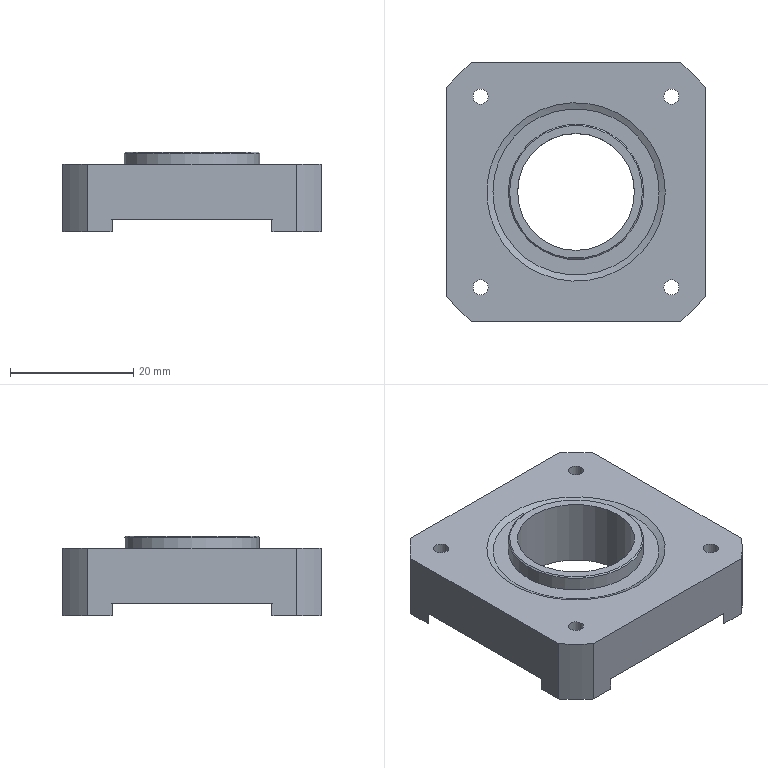Part | NX | 1 solid | 28 faces | box 42 x 42 x 13 mm | volume 13151 mm3 | plane 16 | cylinder 10 | cone 2 | commonest cylinder face diameters 2.459 x4 54 x4 19 x1 22 x1
STEP:
#1=CARTESIAN_POINT('',(-9.5,0.,2.));
#2=VERTEX_POINT('',#1);
#3=CARTESIAN_POINT('',(0.,0.,2.));
#4=DIRECTION('',(0.,0.,-1.));
#5=DIRECTION('',(-1.,0.,0.));
#6=AXIS2_PLACEMENT_3D('',#3,#4,#5);
#7=CIRCLE('',#6,9.5);
#8=EDGE_CURVE('',#2,#2,#7,.T.);
#9=ORIENTED_EDGE('',*,*,#8,.F.);
#10=EDGE_LOOP('',(#9));
#11=FACE_BOUND('',#10,.T.);
#12=CARTESIAN_POINT('',(16.73,-15.5,2.));
#13=VERTEX_POINT('',#12);
#14=CARTESIAN_POINT('',(15.5,-15.5,2.));
#15=DIRECTION('',(0.,0.,1.));
#16=DIRECTION('',(1.,0.,0.));
#17=AXIS2_PLACEMENT_3D('',#14,#15,#16);
#18=CIRCLE('',#17,1.23);
#19=EDGE_CURVE('',#13,#13,#18,.F.);
#20=ORIENTED_EDGE('',*,*,#19,.F.);
#21=EDGE_LOOP('',(#20));
#22=FACE_BOUND('',#21,.T.);
#23=CARTESIAN_POINT('',(-14.271,-15.5,2.));
#24=VERTEX_POINT('',#23);
#25=CARTESIAN_POINT('',(-15.5,-15.5,2.));
#26=DIRECTION('',(0.,0.,1.));
#27=DIRECTION('',(1.,0.,0.));
#28=AXIS2_PLACEMENT_3D('',#25,#26,#27);
#29=CIRCLE('',#28,1.23);
#30=EDGE_CURVE('',#24,#24,#29,.F.);
#31=ORIENTED_EDGE('',*,*,#30,.F.);
#32=EDGE_LOOP('',(#31));
#33=FACE_BOUND('',#32,.T.);
#34=CARTESIAN_POINT('',(16.73,15.5,2.));
#35=VERTEX_POINT('',#34);
#36=CARTESIAN_POINT('',(15.5,15.5,2.));
#37=DIRECTION('',(0.,0.,1.));
#38=DIRECTION('',(1.,0.,0.));
#39=AXIS2_PLACEMENT_3D('',#36,#37,#38);
#40=CIRCLE('',#39,1.23);
#41=EDGE_CURVE('',#35,#35,#40,.F.);
#42=ORIENTED_EDGE('',*,*,#41,.F.);
#43=EDGE_LOOP('',(#42));
#44=FACE_BOUND('',#43,.T.);
#45=CARTESIAN_POINT('',(-14.271,15.5,2.));
#46=VERTEX_POINT('',#45);
#47=CARTESIAN_POINT('',(-15.5,15.5,2.));
#48=DIRECTION('',(0.,0.,1.));
#49=DIRECTION('',(1.,0.,0.));
#50=AXIS2_PLACEMENT_3D('',#47,#48,#49);
#51=CIRCLE('',#50,1.23);
#52=EDGE_CURVE('',#46,#46,#51,.F.);
#53=ORIENTED_EDGE('',*,*,#52,.F.);
#54=EDGE_LOOP('',(#53));
#55=FACE_BOUND('',#54,.T.);
#56=CARTESIAN_POINT('',(13.,-21.,2.));
#57=VERTEX_POINT('',#56);
#58=CARTESIAN_POINT('',(21.,-13.,2.));
#59=VERTEX_POINT('',#58);
#60=CARTESIAN_POINT('',(13.,-21.,2.));
#61=DIRECTION('',(0.7071,0.7071,0.));
#62=VECTOR('',#61,1000.);
#63=LINE('',#60,#62);
#64=EDGE_CURVE('',#57,#59,#63,.T.);
#65=ORIENTED_EDGE('',*,*,#64,.F.);
#66=CARTESIAN_POINT('',(-13.,-21.,2.));
#67=VERTEX_POINT('',#66);
#68=CARTESIAN_POINT('',(0.,-21.,2.));
#69=DIRECTION('',(1.,0.,0.));
#70=VECTOR('',#69,1000.);
#71=LINE('',#68,#70);
#72=EDGE_CURVE('',#67,#57,#71,.T.);
#73=ORIENTED_EDGE('',*,*,#72,.F.);
#74=CARTESIAN_POINT('',(-21.,-13.,2.));
#75=VERTEX_POINT('',#74);
#76=CARTESIAN_POINT('',(-21.,-13.,2.));
#77=DIRECTION('',(0.7071,-0.7071,0.));
#78=VECTOR('',#77,1000.);
#79=LINE('',#76,#78);
#80=EDGE_CURVE('',#75,#67,#79,.T.);
#81=ORIENTED_EDGE('',*,*,#80,.F.);
#82=CARTESIAN_POINT('',(-21.,13.,2.));
#83=VERTEX_POINT('',#82);
#84=CARTESIAN_POINT('',(-21.,0.,2.));
#85=DIRECTION('',(0.,1.,0.));
#86=VECTOR('',#85,1000.);
#87=LINE('',#84,#86);
#88=EDGE_CURVE('',#83,#75,#87,.F.);
#89=ORIENTED_EDGE('',*,*,#88,.F.);
#90=CARTESIAN_POINT('',(-13.,21.,2.));
#91=VERTEX_POINT('',#90);
#92=CARTESIAN_POINT('',(-13.,21.,2.));
#93=DIRECTION('',(-0.7071,-0.7071,0.));
#94=VECTOR('',#93,1000.);
#95=LINE('',#92,#94);
#96=EDGE_CURVE('',#91,#83,#95,.T.);
#97=ORIENTED_EDGE('',*,*,#96,.F.);
#98=CARTESIAN_POINT('',(13.,21.,2.));
#99=VERTEX_POINT('',#98);
#100=CARTESIAN_POINT('',(0.,21.,2.));
#101=DIRECTION('',(1.,0.,0.));
#102=VECTOR('',#101,1000.);
#103=LINE('',#100,#102);
#104=EDGE_CURVE('',#99,#91,#103,.F.);
#105=ORIENTED_EDGE('',*,*,#104,.F.);
#106=CARTESIAN_POINT('',(21.,13.,2.));
#107=VERTEX_POINT('',#106);
#108=CARTESIAN_POINT('',(21.,13.,2.));
#109=DIRECTION('',(-0.7071,0.7071,0.));
#110=VECTOR('',#109,1000.);
#111=LINE('',#108,#110);
#112=EDGE_CURVE('',#107,#99,#111,.T.);
#113=ORIENTED_EDGE('',*,*,#112,.F.);
#114=CARTESIAN_POINT('',(21.,0.,2.));
#115=DIRECTION('',(0.,1.,0.));
#116=VECTOR('',#115,1000.);
#117=LINE('',#114,#116);
#118=EDGE_CURVE('',#59,#107,#117,.T.);
#119=ORIENTED_EDGE('',*,*,#118,.F.);
#120=EDGE_LOOP('',(#65,#73,#81,#89,#97,#105,#113,#119));
#121=FACE_BOUND('',#120,.T.);
#122=CARTESIAN_POINT('',(0.,0.,2.));
#123=DIRECTION('',(0.,0.,1.));
#124=DIRECTION('',(1.,0.,0.));
#125=AXIS2_PLACEMENT_3D('',#122,#123,#124);
#126=PLANE('',#125);
#127=ADVANCED_FACE('',(#11,#22,#33,#44,#55,#121),#126,.F.);
#128=CARTESIAN_POINT('',(-9.5,0.,13.));
#129=VERTEX_POINT('',#128);
#130=CARTESIAN_POINT('',(0.,0.,13.));
#131=DIRECTION('',(0.,0.,-1.));
#132=DIRECTION('',(-1.,0.,0.));
#133=AXIS2_PLACEMENT_3D('',#130,#131,#132);
#134=CIRCLE('',#133,9.5);
#135=EDGE_CURVE('',#129,#129,#134,.T.);
#136=ORIENTED_EDGE('',*,*,#135,.F.);
#137=EDGE_LOOP('',(#136));
#138=FACE_BOUND('',#137,.T.);
#139=ORIENTED_EDGE('',*,*,#8,.T.);
#140=EDGE_LOOP('',(#139));
#141=FACE_BOUND('',#140,.T.);
#142=CARTESIAN_POINT('',(0.,0.,13.));
#143=DIRECTION('',(0.,0.,-1.));
#144=DIRECTION('',(-1.,0.,0.));
#145=AXIS2_PLACEMENT_3D('',#142,#143,#144);
#146=CYLINDRICAL_SURFACE('',#145,9.5);
#147=ADVANCED_FACE('',(#138,#141),#146,.F.);
#148=CARTESIAN_POINT('',(16.73,-15.5,11.));
#149=VERTEX_POINT('',#148);
#150=CARTESIAN_POINT('',(15.5,-15.5,11.));
#151=DIRECTION('',(0.,0.,1.));
#152=DIRECTION('',(1.,0.,0.));
#153=AXIS2_PLACEMENT_3D('',#150,#151,#152);
#154=CIRCLE('',#153,1.23);
#155=EDGE_CURVE('',#149,#149,#154,.F.);
#156=ORIENTED_EDGE('',*,*,#155,.F.);
#157=EDGE_LOOP('',(#156));
#158=FACE_BOUND('',#157,.T.);
#159=ORIENTED_EDGE('',*,*,#19,.T.);
#160=EDGE_LOOP('',(#159));
#161=FACE_BOUND('',#160,.T.);
#162=CARTESIAN_POINT('',(15.5,-15.5,9.75));
#163=DIRECTION('',(0.,0.,1.));
#164=DIRECTION('',(1.,0.,0.));
#165=AXIS2_PLACEMENT_3D('',#162,#163,#164);
#166=CYLINDRICAL_SURFACE('',#165,1.23);
#167=ADVANCED_FACE('',(#158,#161),#166,.F.);
#168=CARTESIAN_POINT('',(-14.271,-15.5,11.));
#169=VERTEX_POINT('',#168);
#170=CARTESIAN_POINT('',(-15.5,-15.5,11.));
#171=DIRECTION('',(0.,0.,1.));
#172=DIRECTION('',(1.,0.,0.));
#173=AXIS2_PLACEMENT_3D('',#170,#171,#172);
#174=CIRCLE('',#173,1.23);
#175=EDGE_CURVE('',#169,#169,#174,.F.);
#176=ORIENTED_EDGE('',*,*,#175,.F.);
#177=EDGE_LOOP('',(#176));
#178=FACE_BOUND('',#177,.T.);
#179=ORIENTED_EDGE('',*,*,#30,.T.);
#180=EDGE_LOOP('',(#179));
#181=FACE_BOUND('',#180,.T.);
#182=CARTESIAN_POINT('',(-15.5,-15.5,9.75));
#183=DIRECTION('',(0.,0.,1.));
#184=DIRECTION('',(1.,0.,0.));
#185=AXIS2_PLACEMENT_3D('',#182,#183,#184);
#186=CYLINDRICAL_SURFACE('',#185,1.23);
#187=ADVANCED_FACE('',(#178,#181),#186,.F.);
#188=CARTESIAN_POINT('',(16.73,15.5,11.));
#189=VERTEX_POINT('',#188);
#190=CARTESIAN_POINT('',(15.5,15.5,11.));
#191=DIRECTION('',(0.,0.,1.));
#192=DIRECTION('',(1.,0.,0.));
#193=AXIS2_PLACEMENT_3D('',#190,#191,#192);
#194=CIRCLE('',#193,1.23);
#195=EDGE_CURVE('',#189,#189,#194,.F.);
#196=ORIENTED_EDGE('',*,*,#195,.F.);
#197=EDGE_LOOP('',(#196));
#198=FACE_BOUND('',#197,.T.);
#199=ORIENTED_EDGE('',*,*,#41,.T.);
#200=EDGE_LOOP('',(#199));
#201=FACE_BOUND('',#200,.T.);
#202=CARTESIAN_POINT('',(15.5,15.5,9.75));
#203=DIRECTION('',(0.,0.,1.));
#204=DIRECTION('',(1.,0.,0.));
#205=AXIS2_PLACEMENT_3D('',#202,#203,#204);
#206=CYLINDRICAL_SURFACE('',#205,1.23);
#207=ADVANCED_FACE('',(#198,#201),#206,.F.);
#208=CARTESIAN_POINT('',(-14.271,15.5,11.));
#209=VERTEX_POINT('',#208);
#210=CARTESIAN_POINT('',(-15.5,15.5,11.));
#211=DIRECTION('',(0.,0.,1.));
#212=DIRECTION('',(1.,0.,0.));
#213=AXIS2_PLACEMENT_3D('',#210,#211,#212);
#214=CIRCLE('',#213,1.23);
#215=EDGE_CURVE('',#209,#209,#214,.F.);
#216=ORIENTED_EDGE('',*,*,#215,.F.);
#217=EDGE_LOOP('',(#216));
#218=FACE_BOUND('',#217,.T.);
#219=ORIENTED_EDGE('',*,*,#52,.T.);
#220=EDGE_LOOP('',(#219));
#221=FACE_BOUND('',#220,.T.);
#222=CARTESIAN_POINT('',(-15.5,15.5,9.75));
#223=DIRECTION('',(0.,0.,1.));
#224=DIRECTION('',(1.,0.,0.));
#225=AXIS2_PLACEMENT_3D('',#222,#223,#224);
#226=CYLINDRICAL_SURFACE('',#225,1.23);
#227=ADVANCED_FACE('',(#218,#221),#226,.F.);
#228=CARTESIAN_POINT('',(21.,-16.971,11.));
#229=VERTEX_POINT('',#228);
#230=CARTESIAN_POINT('',(21.,-16.971,0.));
#231=VERTEX_POINT('',#230);
#232=CARTESIAN_POINT('',(21.,-16.971,0.));
#233=DIRECTION('',(0.,0.,-1.));
#234=VECTOR('',#233,1000.);
#235=LINE('',#232,#234);
#236=EDGE_CURVE('',#229,#231,#235,.T.);
#237=ORIENTED_EDGE('',*,*,#236,.T.);
#238=CARTESIAN_POINT('',(21.,-13.,0.));
#239=VERTEX_POINT('',#238);
#240=CARTESIAN_POINT('',(21.,16.971,0.));
#241=DIRECTION('',(0.,1.,0.));
#242=VECTOR('',#241,1000.);
#243=LINE('',#240,#242);
#244=EDGE_CURVE('',#231,#239,#243,.T.);
#245=ORIENTED_EDGE('',*,*,#244,.T.);
#246=CARTESIAN_POINT('',(21.,-13.,0.));
#247=DIRECTION('',(0.,0.,-1.));
#248=VECTOR('',#247,1000.);
#249=LINE('',#246,#248);
#250=EDGE_CURVE('',#239,#59,#249,.F.);
#251=ORIENTED_EDGE('',*,*,#250,.T.);
#252=ORIENTED_EDGE('',*,*,#118,.T.);
#253=CARTESIAN_POINT('',(21.,13.,0.));
#254=VERTEX_POINT('',#253);
#255=CARTESIAN_POINT('',(21.,13.,0.));
#256=DIRECTION('',(0.,0.,-1.));
#257=VECTOR('',#256,1000.);
#258=LINE('',#255,#257);
#259=EDGE_CURVE('',#107,#254,#258,.T.);
#260=ORIENTED_EDGE('',*,*,#259,.T.);
#261=CARTESIAN_POINT('',(21.,16.971,0.));
#262=VERTEX_POINT('',#261);
#263=CARTESIAN_POINT('',(21.,16.971,0.));
#264=DIRECTION('',(0.,1.,0.));
#265=VECTOR('',#264,1000.);
#266=LINE('',#263,#265);
#267=EDGE_CURVE('',#254,#262,#266,.T.);
#268=ORIENTED_EDGE('',*,*,#267,.T.);
#269=CARTESIAN_POINT('',(21.,16.971,11.));
#270=VERTEX_POINT('',#269);
#271=CARTESIAN_POINT('',(21.,16.971,0.));
#272=DIRECTION('',(0.,0.,-1.));
#273=VECTOR('',#272,1000.);
#274=LINE('',#271,#273);
#275=EDGE_CURVE('',#262,#270,#274,.F.);
#276=ORIENTED_EDGE('',*,*,#275,.T.);
#277=CARTESIAN_POINT('',(21.,16.971,11.));
#278=DIRECTION('',(0.,1.,0.));
#279=VECTOR('',#278,1000.);
#280=LINE('',#277,#279);
#281=EDGE_CURVE('',#270,#229,#280,.F.);
#282=ORIENTED_EDGE('',*,*,#281,.T.);
#283=EDGE_LOOP('',(#237,#245,#251,#252,#260,#268,#276,#282));
#284=FACE_BOUND('',#283,.T.);
#285=CARTESIAN_POINT('',(21.,16.971,0.));
#286=DIRECTION('',(1.,0.,0.));
#287=DIRECTION('',(0.,0.,-1.));
#288=AXIS2_PLACEMENT_3D('',#285,#286,#287);
#289=PLANE('',#288);
#290=ADVANCED_FACE('',(#284),#289,.T.);
#291=ORIENTED_EDGE('',*,*,#250,.F.);
#292=CARTESIAN_POINT('',(13.,-21.,0.));
#293=VERTEX_POINT('',#292);
#294=CARTESIAN_POINT('',(21.,-13.,0.));
#295=DIRECTION('',(0.7071,0.7071,0.));
#296=VECTOR('',#295,1000.);
#297=LINE('',#294,#296);
#298=EDGE_CURVE('',#293,#239,#297,.T.);
#299=ORIENTED_EDGE('',*,*,#298,.F.);
#300=CARTESIAN_POINT('',(13.,-21.,0.));
#301=DIRECTION('',(0.,0.,1.));
#302=VECTOR('',#301,1000.);
#303=LINE('',#300,#302);
#304=EDGE_CURVE('',#57,#293,#303,.F.);
#305=ORIENTED_EDGE('',*,*,#304,.F.);
#306=ORIENTED_EDGE('',*,*,#64,.T.);
#307=EDGE_LOOP('',(#291,#299,#305,#306));
#308=FACE_BOUND('',#307,.T.);
#309=CARTESIAN_POINT('',(21.,-13.,0.));
#310=DIRECTION('',(0.7071,-0.7071,0.));
#311=DIRECTION('',(0.7071,0.7071,0.));
#312=AXIS2_PLACEMENT_3D('',#309,#310,#311);
#313=PLANE('',#312);
#314=ADVANCED_FACE('',(#308),#313,.F.);
#315=CARTESIAN_POINT('',(-13.,-21.,0.));
#316=VERTEX_POINT('',#315);
#317=CARTESIAN_POINT('',(-13.,-21.,0.));
#318=DIRECTION('',(0.,0.,-1.));
#319=VECTOR('',#318,1000.);
#320=LINE('',#317,#319);
#321=EDGE_CURVE('',#316,#67,#320,.F.);
#322=ORIENTED_EDGE('',*,*,#321,.T.);
#323=ORIENTED_EDGE('',*,*,#72,.T.);
#324=ORIENTED_EDGE('',*,*,#304,.T.);
#325=CARTESIAN_POINT('',(16.971,-21.,0.));
#326=VERTEX_POINT('',#325);
#327=CARTESIAN_POINT('',(16.971,-21.,0.));
#328=DIRECTION('',(1.,0.,0.));
#329=VECTOR('',#328,1000.);
#330=LINE('',#327,#329);
#331=EDGE_CURVE('',#293,#326,#330,.T.);
#332=ORIENTED_EDGE('',*,*,#331,.T.);
#333=CARTESIAN_POINT('',(16.971,-21.,11.));
#334=VERTEX_POINT('',#333);
#335=CARTESIAN_POINT('',(16.971,-21.,0.));
#336=DIRECTION('',(0.,0.,-1.));
#337=VECTOR('',#336,1000.);
#338=LINE('',#335,#337);
#339=EDGE_CURVE('',#326,#334,#338,.F.);
#340=ORIENTED_EDGE('',*,*,#339,.T.);
#341=CARTESIAN_POINT('',(-16.971,-21.,11.));
#342=VERTEX_POINT('',#341);
#343=CARTESIAN_POINT('',(16.971,-21.,11.));
#344=DIRECTION('',(1.,0.,0.));
#345=VECTOR('',#344,1000.);
#346=LINE('',#343,#345);
#347=EDGE_CURVE('',#334,#342,#346,.F.);
#348=ORIENTED_EDGE('',*,*,#347,.T.);
#349=CARTESIAN_POINT('',(-16.971,-21.,0.));
#350=VERTEX_POINT('',#349);
#351=CARTESIAN_POINT('',(-16.971,-21.,0.));
#352=DIRECTION('',(0.,0.,-1.));
#353=VECTOR('',#352,1000.);
#354=LINE('',#351,#353);
#355=EDGE_CURVE('',#342,#350,#354,.T.);
#356=ORIENTED_EDGE('',*,*,#355,.T.);
#357=CARTESIAN_POINT('',(16.971,-21.,0.));
#358=DIRECTION('',(1.,0.,0.));
#359=VECTOR('',#358,1000.);
#360=LINE('',#357,#359);
#361=EDGE_CURVE('',#350,#316,#360,.T.);
#362=ORIENTED_EDGE('',*,*,#361,.T.);
#363=EDGE_LOOP('',(#322,#323,#324,#332,#340,#348,#356,#362));
#364=FACE_BOUND('',#363,.T.);
#365=CARTESIAN_POINT('',(16.971,-21.,0.));
#366=DIRECTION('',(0.,-1.,0.));
#367=DIRECTION('',(0.,0.,-1.));
#368=AXIS2_PLACEMENT_3D('',#365,#366,#367);
#369=PLANE('',#368);
#370=ADVANCED_FACE('',(#364),#369,.T.);
#371=ORIENTED_EDGE('',*,*,#321,.F.);
#372=CARTESIAN_POINT('',(-21.,-13.,0.));
#373=VERTEX_POINT('',#372);
#374=CARTESIAN_POINT('',(-13.,-21.,0.));
#375=DIRECTION('',(0.7071,-0.7071,0.));
#376=VECTOR('',#375,1000.);
#377=LINE('',#374,#376);
#378=EDGE_CURVE('',#373,#316,#377,.T.);
#379=ORIENTED_EDGE('',*,*,#378,.F.);
#380=CARTESIAN_POINT('',(-21.,-13.,0.));
#381=DIRECTION('',(0.,0.,1.));
#382=VECTOR('',#381,1000.);
#383=LINE('',#380,#382);
#384=EDGE_CURVE('',#75,#373,#383,.F.);
#385=ORIENTED_EDGE('',*,*,#384,.F.);
#386=ORIENTED_EDGE('',*,*,#80,.T.);
#387=EDGE_LOOP('',(#371,#379,#385,#386));
#388=FACE_BOUND('',#387,.T.);
#389=CARTESIAN_POINT('',(-13.,-21.,0.));
#390=DIRECTION('',(-0.7071,-0.7071,0.));
#391=DIRECTION('',(0.7071,-0.7071,0.));
#392=AXIS2_PLACEMENT_3D('',#389,#390,#391);
#393=PLANE('',#392);
#394=ADVANCED_FACE('',(#388),#393,.F.);
#395=CARTESIAN_POINT('',(-21.,13.,0.));
#396=VERTEX_POINT('',#395);
#397=CARTESIAN_POINT('',(-21.,13.,0.));
#398=DIRECTION('',(0.,0.,1.));
#399=VECTOR('',#398,1000.);
#400=LINE('',#397,#399);
#401=EDGE_CURVE('',#396,#83,#400,.T.);
#402=ORIENTED_EDGE('',*,*,#401,.T.);
#403=ORIENTED_EDGE('',*,*,#88,.T.);
#404=ORIENTED_EDGE('',*,*,#384,.T.);
#405=CARTESIAN_POINT('',(-21.,-16.971,0.));
#406=VERTEX_POINT('',#405);
#407=CARTESIAN_POINT('',(-21.,-16.971,0.));
#408=DIRECTION('',(0.,1.,0.));
#409=VECTOR('',#408,1000.);
#410=LINE('',#407,#409);
#411=EDGE_CURVE('',#373,#406,#410,.F.);
#412=ORIENTED_EDGE('',*,*,#411,.T.);
#413=CARTESIAN_POINT('',(-21.,-16.971,11.));
#414=VERTEX_POINT('',#413);
#415=CARTESIAN_POINT('',(-21.,-16.971,0.));
#416=DIRECTION('',(0.,0.,1.));
#417=VECTOR('',#416,1000.);
#418=LINE('',#415,#417);
#419=EDGE_CURVE('',#406,#414,#418,.T.);
#420=ORIENTED_EDGE('',*,*,#419,.T.);
#421=CARTESIAN_POINT('',(-21.,16.971,11.));
#422=VERTEX_POINT('',#421);
#423=CARTESIAN_POINT('',(-21.,-16.971,11.));
#424=DIRECTION('',(0.,1.,0.));
#425=VECTOR('',#424,1000.);
#426=LINE('',#423,#425);
#427=EDGE_CURVE('',#414,#422,#426,.T.);
#428=ORIENTED_EDGE('',*,*,#427,.T.);
#429=CARTESIAN_POINT('',(-21.,16.971,0.));
#430=VERTEX_POINT('',#429);
#431=CARTESIAN_POINT('',(-21.,16.971,0.));
#432=DIRECTION('',(0.,0.,1.));
#433=VECTOR('',#432,1000.);
#434=LINE('',#431,#433);
#435=EDGE_CURVE('',#422,#430,#434,.F.);
#436=ORIENTED_EDGE('',*,*,#435,.T.);
#437=CARTESIAN_POINT('',(-21.,-16.971,0.));
#438=DIRECTION('',(0.,1.,0.));
#439=VECTOR('',#438,1000.);
#440=LINE('',#437,#439);
#441=EDGE_CURVE('',#430,#396,#440,.F.);
#442=ORIENTED_EDGE('',*,*,#441,.T.);
#443=EDGE_LOOP('',(#402,#403,#404,#412,#420,#428,#436,#442));
#444=FACE_BOUND('',#443,.T.);
#445=CARTESIAN_POINT('',(-21.,-16.971,0.));
#446=DIRECTION('',(-1.,0.,0.));
#447=DIRECTION('',(0.,0.,1.));
#448=AXIS2_PLACEMENT_3D('',#445,#446,#447);
#449=PLANE('',#448);
#450=ADVANCED_FACE('',(#444),#449,.T.);
#451=ORIENTED_EDGE('',*,*,#401,.F.);
#452=CARTESIAN_POINT('',(-13.,21.,0.));
#453=VERTEX_POINT('',#452);
#454=CARTESIAN_POINT('',(-21.,13.,0.));
#455=DIRECTION('',(-0.7071,-0.7071,0.));
#456=VECTOR('',#455,1000.);
#457=LINE('',#454,#456);
#458=EDGE_CURVE('',#453,#396,#457,.T.);
#459=ORIENTED_EDGE('',*,*,#458,.F.);
#460=CARTESIAN_POINT('',(-13.,21.,0.));
#461=DIRECTION('',(0.,0.,1.));
#462=VECTOR('',#461,1000.);
#463=LINE('',#460,#462);
#464=EDGE_CURVE('',#91,#453,#463,.F.);
#465=ORIENTED_EDGE('',*,*,#464,.F.);
#466=ORIENTED_EDGE('',*,*,#96,.T.);
#467=EDGE_LOOP('',(#451,#459,#465,#466));
#468=FACE_BOUND('',#467,.T.);
#469=CARTESIAN_POINT('',(-21.,13.,0.));
#470=DIRECTION('',(-0.7071,0.7071,0.));
#471=DIRECTION('',(-0.7071,-0.7071,0.));
#472=AXIS2_PLACEMENT_3D('',#469,#470,#471);
#473=PLANE('',#472);
#474=ADVANCED_FACE('',(#468),#473,.F.);
#475=CARTESIAN_POINT('',(16.971,21.,11.));
#476=VERTEX_POINT('',#475);
#477=CARTESIAN_POINT('',(16.971,21.,0.));
#478=VERTEX_POINT('',#477);
#479=CARTESIAN_POINT('',(16.971,21.,0.));
#480=DIRECTION('',(0.,0.,1.));
#481=VECTOR('',#480,1000.);
#482=LINE('',#479,#481);
#483=EDGE_CURVE('',#476,#478,#482,.F.);
#484=ORIENTED_EDGE('',*,*,#483,.T.);
#485=CARTESIAN_POINT('',(13.,21.,0.));
#486=VERTEX_POINT('',#485);
#487=CARTESIAN_POINT('',(-16.971,21.,0.));
#488=DIRECTION('',(1.,0.,0.));
#489=VECTOR('',#488,1000.);
#490=LINE('',#487,#489);
#491=EDGE_CURVE('',#478,#486,#490,.F.);
#492=ORIENTED_EDGE('',*,*,#491,.T.);
#493=CARTESIAN_POINT('',(13.,21.,0.));
#494=DIRECTION('',(0.,0.,1.));
#495=VECTOR('',#494,1000.);
#496=LINE('',#493,#495);
#497=EDGE_CURVE('',#486,#99,#496,.T.);
#498=ORIENTED_EDGE('',*,*,#497,.T.);
#499=ORIENTED_EDGE('',*,*,#104,.T.);
#500=ORIENTED_EDGE('',*,*,#464,.T.);
#501=CARTESIAN_POINT('',(-16.971,21.,0.));
#502=VERTEX_POINT('',#501);
#503=CARTESIAN_POINT('',(-16.971,21.,0.));
#504=DIRECTION('',(1.,0.,0.));
#505=VECTOR('',#504,1000.);
#506=LINE('',#503,#505);
#507=EDGE_CURVE('',#453,#502,#506,.F.);
#508=ORIENTED_EDGE('',*,*,#507,.T.);
#509=CARTESIAN_POINT('',(-16.971,21.,11.));
#510=VERTEX_POINT('',#509);
#511=CARTESIAN_POINT('',(-16.971,21.,0.));
#512=DIRECTION('',(0.,0.,1.));
#513=VECTOR('',#512,1000.);
#514=LINE('',#511,#513);
#515=EDGE_CURVE('',#502,#510,#514,.T.);
#516=ORIENTED_EDGE('',*,*,#515,.T.);
#517=CARTESIAN_POINT('',(-16.971,21.,11.));
#518=DIRECTION('',(1.,0.,0.));
#519=VECTOR('',#518,1000.);
#520=LINE('',#517,#519);
#521=EDGE_CURVE('',#510,#476,#520,.T.);
#522=ORIENTED_EDGE('',*,*,#521,.T.);
#523=EDGE_LOOP('',(#484,#492,#498,#499,#500,#508,#516,#522));
#524=FACE_BOUND('',#523,.T.);
#525=CARTESIAN_POINT('',(-16.971,21.,0.));
#526=DIRECTION('',(0.,1.,0.));
#527=DIRECTION('',(0.,0.,1.));
#528=AXIS2_PLACEMENT_3D('',#525,#526,#527);
#529=PLANE('',#528);
#530=ADVANCED_FACE('',(#524),#529,.T.);
#531=ORIENTED_EDGE('',*,*,#497,.F.);
#532=CARTESIAN_POINT('',(13.,21.,0.));
#533=DIRECTION('',(-0.7071,0.7071,0.));
#534=VECTOR('',#533,1000.);
#535=LINE('',#532,#534);
#536=EDGE_CURVE('',#254,#486,#535,.T.);
#537=ORIENTED_EDGE('',*,*,#536,.F.);
#538=ORIENTED_EDGE('',*,*,#259,.F.);
#539=ORIENTED_EDGE('',*,*,#112,.T.);
#540=EDGE_LOOP('',(#531,#537,#538,#539));
#541=FACE_BOUND('',#540,.T.);
#542=CARTESIAN_POINT('',(13.,21.,0.));
#543=DIRECTION('',(0.7071,0.7071,0.));
#544=DIRECTION('',(-0.7071,0.7071,0.));
#545=AXIS2_PLACEMENT_3D('',#542,#543,#544);
#546=PLANE('',#545);
#547=ADVANCED_FACE('',(#541),#546,.F.);
#548=ORIENTED_EDGE('',*,*,#135,.T.);
#549=EDGE_LOOP('',(#548));
#550=FACE_BOUND('',#549,.T.);
#551=CARTESIAN_POINT('',(-10.8,0.,13.));
#552=VERTEX_POINT('',#551);
#553=CARTESIAN_POINT('',(0.,0.,13.));
#554=DIRECTION('',(0.,0.,-1.));
#555=DIRECTION('',(-1.,0.,0.));
#556=AXIS2_PLACEMENT_3D('',#553,#554,#555);
#557=CIRCLE('',#556,10.8);
#558=EDGE_CURVE('',#552,#552,#557,.T.);
#559=ORIENTED_EDGE('',*,*,#558,.F.);
#560=EDGE_LOOP('',(#559));
#561=FACE_BOUND('',#560,.T.);
#562=CARTESIAN_POINT('',(0.,0.,13.));
#563=DIRECTION('',(0.,0.,-1.));
#564=DIRECTION('',(-1.,0.,0.));
#565=AXIS2_PLACEMENT_3D('',#562,#563,#564);
#566=PLANE('',#565);
#567=ADVANCED_FACE('',(#550,#561),#566,.F.);
#568=CARTESIAN_POINT('',(14.5,0.,11.));
#569=VERTEX_POINT('',#568);
#570=CARTESIAN_POINT('',(0.,0.,11.));
#571=DIRECTION('',(0.,0.,1.));
#572=DIRECTION('',(1.,0.,0.));
#573=AXIS2_PLACEMENT_3D('',#570,#571,#572);
#574=CIRCLE('',#573,14.5);
#575=EDGE_CURVE('',#569,#569,#574,.F.);
#576=ORIENTED_EDGE('',*,*,#575,.T.);
#577=EDGE_LOOP('',(#576));
#578=FACE_BOUND('',#577,.T.);
#579=ORIENTED_EDGE('',*,*,#175,.T.);
#580=EDGE_LOOP('',(#579));
#581=FACE_BOUND('',#580,.T.);
#582=ORIENTED_EDGE('',*,*,#155,.T.);
#583=EDGE_LOOP('',(#582));
#584=FACE_BOUND('',#583,.T.);
#585=ORIENTED_EDGE('',*,*,#215,.T.);
#586=EDGE_LOOP('',(#585));
#587=FACE_BOUND('',#586,.T.);
#588=ORIENTED_EDGE('',*,*,#195,.T.);
#589=EDGE_LOOP('',(#588));
#590=FACE_BOUND('',#589,.T.);
#591=ORIENTED_EDGE('',*,*,#281,.F.);
#592=CARTESIAN_POINT('',(0.,0.,11.));
#593=DIRECTION('',(0.,0.,1.));
#594=DIRECTION('',(1.,0.,0.));
#595=AXIS2_PLACEMENT_3D('',#592,#593,#594);
#596=CIRCLE('',#595,27.);
#597=EDGE_CURVE('',#270,#476,#596,.T.);
#598=ORIENTED_EDGE('',*,*,#597,.T.);
#599=ORIENTED_EDGE('',*,*,#521,.F.);
#600=CARTESIAN_POINT('',(0.,0.,11.));
#601=DIRECTION('',(0.,0.,1.));
#602=DIRECTION('',(1.,0.,0.));
#603=AXIS2_PLACEMENT_3D('',#600,#601,#602);
#604=CIRCLE('',#603,27.);
#605=EDGE_CURVE('',#510,#422,#604,.T.);
#606=ORIENTED_EDGE('',*,*,#605,.T.);
#607=ORIENTED_EDGE('',*,*,#427,.F.);
#608=CARTESIAN_POINT('',(0.,0.,11.));
#609=DIRECTION('',(0.,0.,1.));
#610=DIRECTION('',(1.,0.,0.));
#611=AXIS2_PLACEMENT_3D('',#608,#609,#610);
#612=CIRCLE('',#611,27.);
#613=EDGE_CURVE('',#414,#342,#612,.T.);
#614=ORIENTED_EDGE('',*,*,#613,.T.);
#615=ORIENTED_EDGE('',*,*,#347,.F.);
#616=CARTESIAN_POINT('',(0.,0.,11.));
#617=DIRECTION('',(0.,0.,1.));
#618=DIRECTION('',(1.,0.,0.));
#619=AXIS2_PLACEMENT_3D('',#616,#617,#618);
#620=CIRCLE('',#619,27.);
#621=EDGE_CURVE('',#334,#229,#620,.T.);
#622=ORIENTED_EDGE('',*,*,#621,.T.);
#623=EDGE_LOOP('',(#591,#598,#599,#606,#607,#614,#615,#622));
#624=FACE_BOUND('',#623,.T.);
#625=CARTESIAN_POINT('',(0.,0.,11.));
#626=DIRECTION('',(0.,0.,1.));
#627=DIRECTION('',(1.,0.,0.));
#628=AXIS2_PLACEMENT_3D('',#625,#626,#627);
#629=PLANE('',#628);
#630=ADVANCED_FACE('',(#578,#581,#584,#587,#590,#624),#629,.T.);
#631=ORIENTED_EDGE('',*,*,#244,.F.);
#632=CARTESIAN_POINT('',(0.,0.,0.));
#633=DIRECTION('',(0.,0.,1.));
#634=DIRECTION('',(1.,0.,0.));
#635=AXIS2_PLACEMENT_3D('',#632,#633,#634);
#636=CIRCLE('',#635,27.);
#637=EDGE_CURVE('',#326,#231,#636,.T.);
#638=ORIENTED_EDGE('',*,*,#637,.F.);
#639=ORIENTED_EDGE('',*,*,#331,.F.);
#640=ORIENTED_EDGE('',*,*,#298,.T.);
#641=EDGE_LOOP('',(#631,#638,#639,#640));
#642=FACE_BOUND('',#641,.T.);
#643=CARTESIAN_POINT('',(0.,0.,0.));
#644=DIRECTION('',(0.,0.,1.));
#645=DIRECTION('',(1.,0.,0.));
#646=AXIS2_PLACEMENT_3D('',#643,#644,#645);
#647=PLANE('',#646);
#648=ADVANCED_FACE('',(#642),#647,.F.);
#649=ORIENTED_EDGE('',*,*,#637,.T.);
#650=ORIENTED_EDGE('',*,*,#236,.F.);
#651=ORIENTED_EDGE('',*,*,#621,.F.);
#652=ORIENTED_EDGE('',*,*,#339,.F.);
#653=EDGE_LOOP('',(#649,#650,#651,#652));
#654=FACE_BOUND('',#653,.T.);
#655=CARTESIAN_POINT('',(0.,0.,0.));
#656=DIRECTION('',(0.,0.,1.));
#657=DIRECTION('',(1.,0.,0.));
#658=AXIS2_PLACEMENT_3D('',#655,#656,#657);
#659=CYLINDRICAL_SURFACE('',#658,27.);
#660=ADVANCED_FACE('',(#654),#659,.T.);
#661=CARTESIAN_POINT('',(0.,0.,0.));
#662=DIRECTION('',(0.,0.,1.));
#663=DIRECTION('',(1.,0.,0.));
#664=AXIS2_PLACEMENT_3D('',#661,#662,#663);
#665=CIRCLE('',#664,27.);
#666=EDGE_CURVE('',#262,#478,#665,.T.);
#667=ORIENTED_EDGE('',*,*,#666,.T.);
#668=ORIENTED_EDGE('',*,*,#483,.F.);
#669=ORIENTED_EDGE('',*,*,#597,.F.);
#670=ORIENTED_EDGE('',*,*,#275,.F.);
#671=EDGE_LOOP('',(#667,#668,#669,#670));
#672=FACE_BOUND('',#671,.T.);
#673=CARTESIAN_POINT('',(0.,0.,0.));
#674=DIRECTION('',(0.,0.,1.));
#675=DIRECTION('',(1.,0.,0.));
#676=AXIS2_PLACEMENT_3D('',#673,#674,#675);
#677=CYLINDRICAL_SURFACE('',#676,27.);
#678=ADVANCED_FACE('',(#672),#677,.T.);
#679=ORIENTED_EDGE('',*,*,#491,.F.);
#680=ORIENTED_EDGE('',*,*,#666,.F.);
#681=ORIENTED_EDGE('',*,*,#267,.F.);
#682=ORIENTED_EDGE('',*,*,#536,.T.);
#683=EDGE_LOOP('',(#679,#680,#681,#682));
#684=FACE_BOUND('',#683,.T.);
#685=CARTESIAN_POINT('',(0.,0.,0.));
#686=DIRECTION('',(0.,0.,1.));
#687=DIRECTION('',(1.,0.,0.));
#688=AXIS2_PLACEMENT_3D('',#685,#686,#687);
#689=PLANE('',#688);
#690=ADVANCED_FACE('',(#684),#689,.F.);
#691=ORIENTED_EDGE('',*,*,#361,.F.);
#692=CARTESIAN_POINT('',(0.,0.,0.));
#693=DIRECTION('',(0.,0.,1.));
#694=DIRECTION('',(1.,0.,0.));
#695=AXIS2_PLACEMENT_3D('',#692,#693,#694);
#696=CIRCLE('',#695,27.);
#697=EDGE_CURVE('',#406,#350,#696,.T.);
#698=ORIENTED_EDGE('',*,*,#697,.F.);
#699=ORIENTED_EDGE('',*,*,#411,.F.);
#700=ORIENTED_EDGE('',*,*,#378,.T.);
#701=EDGE_LOOP('',(#691,#698,#699,#700));
#702=FACE_BOUND('',#701,.T.);
#703=CARTESIAN_POINT('',(0.,0.,0.));
#704=DIRECTION('',(0.,0.,1.));
#705=DIRECTION('',(1.,0.,0.));
#706=AXIS2_PLACEMENT_3D('',#703,#704,#705);
#707=PLANE('',#706);
#708=ADVANCED_FACE('',(#702),#707,.F.);
#709=ORIENTED_EDGE('',*,*,#697,.T.);
#710=ORIENTED_EDGE('',*,*,#355,.F.);
#711=ORIENTED_EDGE('',*,*,#613,.F.);
#712=ORIENTED_EDGE('',*,*,#419,.F.);
#713=EDGE_LOOP('',(#709,#710,#711,#712));
#714=FACE_BOUND('',#713,.T.);
#715=CARTESIAN_POINT('',(0.,0.,0.));
#716=DIRECTION('',(0.,0.,1.));
#717=DIRECTION('',(1.,0.,0.));
#718=AXIS2_PLACEMENT_3D('',#715,#716,#717);
#719=CYLINDRICAL_SURFACE('',#718,27.);
#720=ADVANCED_FACE('',(#714),#719,.T.);
#721=ORIENTED_EDGE('',*,*,#441,.F.);
#722=CARTESIAN_POINT('',(0.,0.,0.));
#723=DIRECTION('',(0.,0.,1.));
#724=DIRECTION('',(1.,0.,0.));
#725=AXIS2_PLACEMENT_3D('',#722,#723,#724);
#726=CIRCLE('',#725,27.);
#727=EDGE_CURVE('',#502,#430,#726,.T.);
#728=ORIENTED_EDGE('',*,*,#727,.F.);
#729=ORIENTED_EDGE('',*,*,#507,.F.);
#730=ORIENTED_EDGE('',*,*,#458,.T.);
#731=EDGE_LOOP('',(#721,#728,#729,#730));
#732=FACE_BOUND('',#731,.T.);
#733=CARTESIAN_POINT('',(0.,0.,0.));
#734=DIRECTION('',(0.,0.,1.));
#735=DIRECTION('',(1.,0.,0.));
#736=AXIS2_PLACEMENT_3D('',#733,#734,#735);
#737=PLANE('',#736);
#738=ADVANCED_FACE('',(#732),#737,.F.);
#739=ORIENTED_EDGE('',*,*,#727,.T.);
#740=ORIENTED_EDGE('',*,*,#435,.F.);
#741=ORIENTED_EDGE('',*,*,#605,.F.);
#742=ORIENTED_EDGE('',*,*,#515,.F.);
#743=EDGE_LOOP('',(#739,#740,#741,#742));
#744=FACE_BOUND('',#743,.T.);
#745=CARTESIAN_POINT('',(0.,0.,0.));
#746=DIRECTION('',(0.,0.,1.));
#747=DIRECTION('',(1.,0.,0.));
#748=AXIS2_PLACEMENT_3D('',#745,#746,#747);
#749=CYLINDRICAL_SURFACE('',#748,27.);
#750=ADVANCED_FACE('',(#744),#749,.T.);
#751=CARTESIAN_POINT('',(11.,0.,12.8));
#752=VERTEX_POINT('',#751);
#753=CARTESIAN_POINT('',(0.,0.,12.8));
#754=DIRECTION('',(0.,0.,-1.));
#755=DIRECTION('',(-1.,0.,0.));
#756=AXIS2_PLACEMENT_3D('',#753,#754,#755);
#757=CIRCLE('',#756,11.);
#758=EDGE_CURVE('',#752,#752,#757,.F.);
#759=ORIENTED_EDGE('',*,*,#758,.T.);
#760=EDGE_LOOP('',(#759));
#761=FACE_BOUND('',#760,.T.);
#762=ORIENTED_EDGE('',*,*,#558,.T.);
#763=EDGE_LOOP('',(#762));
#764=FACE_BOUND('',#763,.T.);
#765=CARTESIAN_POINT('',(0.,0.,12.8));
#766=DIRECTION('',(0.,0.,-1.));
#767=DIRECTION('',(-1.,0.,0.));
#768=AXIS2_PLACEMENT_3D('',#765,#766,#767);
#769=CONICAL_SURFACE('',#768,11.,0.7854);
#770=ADVANCED_FACE('',(#761,#764),#769,.T.);
#771=ORIENTED_EDGE('',*,*,#575,.F.);
#772=EDGE_LOOP('',(#771));
#773=FACE_BOUND('',#772,.T.);
#774=CARTESIAN_POINT('',(13.5,0.,10.5));
#775=VERTEX_POINT('',#774);
#776=CARTESIAN_POINT('',(0.,0.,10.5));
#777=DIRECTION('',(0.,0.,1.));
#778=DIRECTION('',(1.,0.,0.));
#779=AXIS2_PLACEMENT_3D('',#776,#777,#778);
#780=CIRCLE('',#779,13.5);
#781=EDGE_CURVE('',#775,#775,#780,.T.);
#782=ORIENTED_EDGE('',*,*,#781,.F.);
#783=EDGE_LOOP('',(#782));
#784=FACE_BOUND('',#783,.T.);
#785=CARTESIAN_POINT('',(0.,0.,11.));
#786=DIRECTION('',(0.,0.,1.));
#787=DIRECTION('',(1.,0.,0.));
#788=AXIS2_PLACEMENT_3D('',#785,#786,#787);
#789=CONICAL_SURFACE('',#788,14.5,1.107);
#790=ADVANCED_FACE('',(#773,#784),#789,.F.);
#791=ORIENTED_EDGE('',*,*,#758,.F.);
#792=EDGE_LOOP('',(#791));
#793=FACE_BOUND('',#792,.T.);
#794=CARTESIAN_POINT('',(11.,0.,10.5));
#795=VERTEX_POINT('',#794);
#796=CARTESIAN_POINT('',(0.,0.,10.5));
#797=DIRECTION('',(0.,0.,1.));
#798=DIRECTION('',(1.,0.,0.));
#799=AXIS2_PLACEMENT_3D('',#796,#797,#798);
#800=CIRCLE('',#799,11.);
#801=EDGE_CURVE('',#795,#795,#800,.T.);
#802=ORIENTED_EDGE('',*,*,#801,.T.);
#803=EDGE_LOOP('',(#802));
#804=FACE_BOUND('',#803,.T.);
#805=CARTESIAN_POINT('',(0.,0.,11.));
#806=DIRECTION('',(0.,0.,1.));
#807=DIRECTION('',(1.,0.,0.));
#808=AXIS2_PLACEMENT_3D('',#805,#806,#807);
#809=CYLINDRICAL_SURFACE('',#808,11.);
#810=ADVANCED_FACE('',(#793,#804),#809,.T.);
#811=ORIENTED_EDGE('',*,*,#801,.F.);
#812=EDGE_LOOP('',(#811));
#813=FACE_BOUND('',#812,.T.);
#814=ORIENTED_EDGE('',*,*,#781,.T.);
#815=EDGE_LOOP('',(#814));
#816=FACE_BOUND('',#815,.T.);
#817=CARTESIAN_POINT('',(0.,0.,10.5));
#818=DIRECTION('',(0.,0.,-1.));
#819=DIRECTION('',(-1.,0.,0.));
#820=AXIS2_PLACEMENT_3D('',#817,#818,#819);
#821=PLANE('',#820);
#822=ADVANCED_FACE('',(#813,#816),#821,.F.);
#823=CLOSED_SHELL('',(#127,#147,#167,#187,#207,#227,#290,#314,#370,#394,#450,#474,#530,#547,#567,#630,#648,#660,#678,#690,#708,#720,#738,#750,#770,#790,#810,#822));
#824=MANIFOLD_SOLID_BREP('',#823);
#825=(LENGTH_UNIT()NAMED_UNIT(*)SI_UNIT(.MILLI.,.METRE.));
#826=UNCERTAINTY_MEASURE_WITH_UNIT(LENGTH_MEASURE(0.00001),#825,'','');
#827=(NAMED_UNIT(*)PLANE_ANGLE_UNIT()SI_UNIT($,.RADIAN.));
#828=(NAMED_UNIT(*)SI_UNIT($,.STERADIAN.)SOLID_ANGLE_UNIT());
#829=(GEOMETRIC_REPRESENTATION_CONTEXT(3)GLOBAL_UNCERTAINTY_ASSIGNED_CONTEXT((#826))GLOBAL_UNIT_ASSIGNED_CONTEXT((#825,#827,#828))REPRESENTATION_CONTEXT('',''));
#830=ADVANCED_BREP_SHAPE_REPRESENTATION('',(#824),#829);